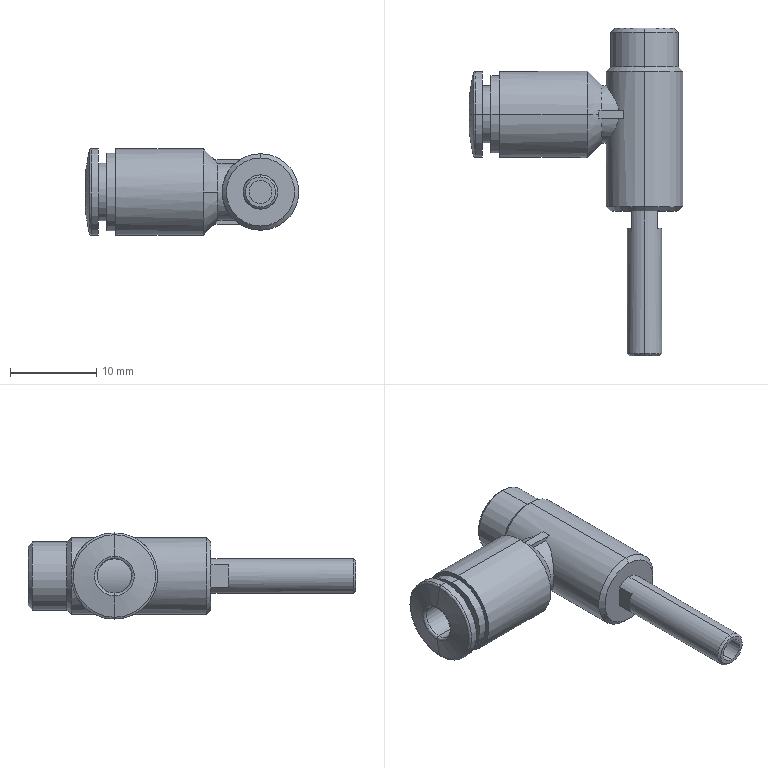Part | STEP file | 1_11 | 1 solid | 62 faces | box 24.75 x 38 x 10 mm | volume 2280 mm3 | cylinder 23 | plane 22 | cone 13 | spline 4 | commonest cylinder face diameters 4 x4 6.667 x4 10 x4 8.9 x3 2.667 x2 6 x2